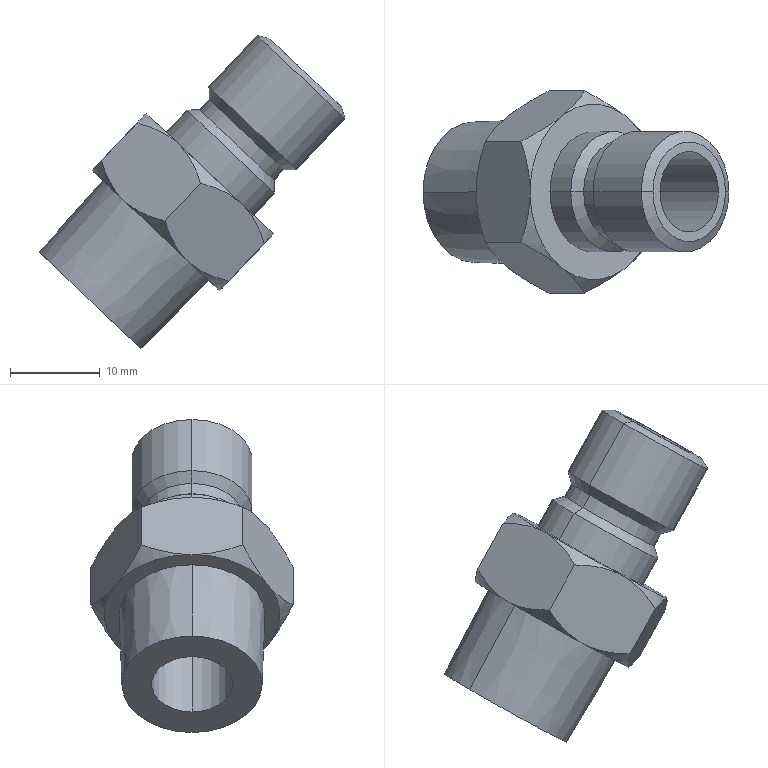Part | STEP file | 4-20.sldasm-Part-51 | 1 solid | 38 faces | box 34.118 x 22.56 x 34.901 mm | volume 4861 mm3 | cone 20 | plane 10 | cylinder 8 | commonest cylinder face diameters 13.462 x4 9 x2 11.43 x2
STEP:
#1=CARTESIAN_POINT('',(267.035,-375.875,53.742));
#2=VERTEX_POINT('',#1);
#3=CARTESIAN_POINT('',(255.664,-375.875,64.491));
#4=VERTEX_POINT('',#3);
#5=CARTESIAN_POINT('',(261.349,-375.875,59.117));
#6=DIRECTION('',(0.687,0.,0.7267));
#7=DIRECTION('',(-0.7267,0.,0.687));
#8=AXIS2_PLACEMENT_3D('',#5,#6,#7);
#9=CIRCLE('',#8,7.824);
#10=EDGE_CURVE('',#2,#4,#9,.T.);
#11=ORIENTED_EDGE('',*,*,#10,.T.);
#12=CARTESIAN_POINT('',(262.798,-375.875,72.445));
#13=VERTEX_POINT('',#12);
#14=CARTESIAN_POINT('',(262.798,-375.875,72.445));
#15=DIRECTION('',(0.6677,0.,0.7444));
#16=VECTOR('',#15,1000.);
#17=LINE('',#14,#16);
#18=EDGE_CURVE('',#4,#13,#17,.T.);
#19=ORIENTED_EDGE('',*,*,#18,.T.);
#20=CARTESIAN_POINT('',(274.575,-375.875,61.312));
#21=VERTEX_POINT('',#20);
#22=CARTESIAN_POINT('',(268.686,-375.875,66.878));
#23=DIRECTION('',(-0.687,0.,-0.7267));
#24=DIRECTION('',(-0.7267,0.,0.687));
#25=AXIS2_PLACEMENT_3D('',#22,#23,#24);
#26=CIRCLE('',#25,8.103);
#27=EDGE_CURVE('',#13,#21,#26,.T.);
#28=ORIENTED_EDGE('',*,*,#27,.T.);
#29=CARTESIAN_POINT('',(274.575,-375.875,61.312));
#30=DIRECTION('',(0.7057,0.,0.7085));
#31=VECTOR('',#30,1000.);
#32=LINE('',#29,#31);
#33=EDGE_CURVE('',#2,#21,#32,.T.);
#34=ORIENTED_EDGE('',*,*,#33,.F.);
#35=EDGE_LOOP('',(#11,#19,#28,#34));
#36=FACE_OUTER_BOUND('',#35,.T.);
#37=CARTESIAN_POINT('',(268.686,-375.875,66.878));
#38=DIRECTION('',(0.687,0.,0.7267));
#39=DIRECTION('',(0.7267,0.,-0.687));
#40=AXIS2_PLACEMENT_3D('',#37,#38,#39);
#41=CONICAL_SURFACE('',#40,8.103,0.02618);
#42=ADVANCED_FACE('',(#36),#41,.T.);
#43=CARTESIAN_POINT('',(289.399,-375.875,80.678));
#44=VERTEX_POINT('',#43);
#45=CARTESIAN_POINT('',(281.301,-375.875,88.334));
#46=VERTEX_POINT('',#45);
#47=CARTESIAN_POINT('',(285.35,-375.875,84.506));
#48=DIRECTION('',(0.687,0.,0.7267));
#49=DIRECTION('',(-0.7267,0.,0.687));
#50=AXIS2_PLACEMENT_3D('',#47,#48,#49);
#51=CIRCLE('',#50,5.572);
#52=EDGE_CURVE('',#44,#46,#51,.T.);
#53=ORIENTED_EDGE('',*,*,#52,.F.);
#54=CARTESIAN_POINT('',(289.781,-375.875,79.396));
#55=VERTEX_POINT('',#54);
#56=CARTESIAN_POINT('',(289.151,-375.875,81.508));
#57=DIRECTION('',(0.2859,0.,-0.9583));
#58=VECTOR('',#57,1000.);
#59=LINE('',#56,#58);
#60=EDGE_CURVE('',#44,#55,#59,.T.);
#61=ORIENTED_EDGE('',*,*,#60,.T.);
#62=CARTESIAN_POINT('',(279.999,-375.875,88.643));
#63=VERTEX_POINT('',#62);
#64=CARTESIAN_POINT('',(284.89,-375.875,84.02));
#65=DIRECTION('',(0.687,0.,0.7267));
#66=DIRECTION('',(-0.7267,0.,0.687));
#67=AXIS2_PLACEMENT_3D('',#64,#65,#66);
#68=CIRCLE('',#67,6.731);
#69=EDGE_CURVE('',#55,#63,#68,.T.);
#70=ORIENTED_EDGE('',*,*,#69,.T.);
#71=CARTESIAN_POINT('',(282.143,-375.875,88.133));
#72=DIRECTION('',(-0.9728,0.,0.2316));
#73=VECTOR('',#72,1000.);
#74=LINE('',#71,#73);
#75=EDGE_CURVE('',#46,#63,#74,.T.);
#76=ORIENTED_EDGE('',*,*,#75,.F.);
#77=EDGE_LOOP('',(#53,#61,#70,#76));
#78=FACE_OUTER_BOUND('',#77,.T.);
#79=CARTESIAN_POINT('',(285.647,-375.875,84.821));
#80=DIRECTION('',(-0.687,0.,-0.7267));
#81=DIRECTION('',(-0.7267,0.,0.687));
#82=AXIS2_PLACEMENT_3D('',#79,#80,#81);
#83=CONICAL_SURFACE('',#82,4.822,1.047);
#84=ADVANCED_FACE('',(#78),#83,.T.);
#85=ORIENTED_EDGE('',*,*,#69,.F.);
#86=CARTESIAN_POINT('',(284.396,-375.875,73.698));
#87=VERTEX_POINT('',#86);
#88=CARTESIAN_POINT('',(266.241,-375.875,54.493));
#89=DIRECTION('',(-0.687,0.,-0.7267));
#90=VECTOR('',#89,1000.);
#91=LINE('',#88,#90);
#92=EDGE_CURVE('',#55,#87,#91,.T.);
#93=ORIENTED_EDGE('',*,*,#92,.T.);
#94=CARTESIAN_POINT('',(274.613,-375.875,82.946));
#95=VERTEX_POINT('',#94);
#96=CARTESIAN_POINT('',(279.504,-375.875,78.322));
#97=DIRECTION('',(0.687,0.,0.7267));
#98=DIRECTION('',(-0.7267,0.,0.687));
#99=AXIS2_PLACEMENT_3D('',#96,#97,#98);
#100=CIRCLE('',#99,6.731);
#101=EDGE_CURVE('',#87,#95,#100,.T.);
#102=ORIENTED_EDGE('',*,*,#101,.T.);
#103=CARTESIAN_POINT('',(256.458,-375.875,63.74));
#104=DIRECTION('',(-0.687,0.,-0.7267));
#105=VECTOR('',#104,1000.);
#106=LINE('',#103,#105);
#107=EDGE_CURVE('',#63,#95,#106,.T.);
#108=ORIENTED_EDGE('',*,*,#107,.F.);
#109=EDGE_LOOP('',(#85,#93,#102,#108));
#110=FACE_OUTER_BOUND('',#109,.T.);
#111=CARTESIAN_POINT('',(261.349,-375.875,59.117));
#112=DIRECTION('',(-0.687,0.,-0.7267));
#113=DIRECTION('',(-0.7267,0.,0.687));
#114=AXIS2_PLACEMENT_3D('',#111,#112,#113);
#115=CYLINDRICAL_SURFACE('',#114,6.731);
#116=ADVANCED_FACE('',(#110),#115,.T.);
#117=CARTESIAN_POINT('',(282.96,-375.875,73.658));
#118=VERTEX_POINT('',#117);
#119=CARTESIAN_POINT('',(274.653,-375.875,81.51));
#120=VERTEX_POINT('',#119);
#121=CARTESIAN_POINT('',(278.806,-375.875,77.584));
#122=DIRECTION('',(0.687,0.,0.7267));
#123=DIRECTION('',(-0.7267,0.,0.687));
#124=AXIS2_PLACEMENT_3D('',#121,#122,#123);
#125=CIRCLE('',#124,5.715);
#126=EDGE_CURVE('',#118,#120,#125,.T.);
#127=ORIENTED_EDGE('',*,*,#126,.T.);
#128=CARTESIAN_POINT('',(274.613,-375.875,82.946));
#129=DIRECTION('',(-0.02811,0.,0.9996));
#130=VECTOR('',#129,1000.);
#131=LINE('',#128,#130);
#132=EDGE_CURVE('',#120,#95,#131,.T.);
#133=ORIENTED_EDGE('',*,*,#132,.T.);
#134=ORIENTED_EDGE('',*,*,#101,.F.);
#135=CARTESIAN_POINT('',(284.396,-375.875,73.698));
#136=DIRECTION('',(0.9996,0.,0.02811));
#137=VECTOR('',#136,1000.);
#138=LINE('',#135,#137);
#139=EDGE_CURVE('',#118,#87,#138,.T.);
#140=ORIENTED_EDGE('',*,*,#139,.F.);
#141=EDGE_LOOP('',(#127,#133,#134,#140));
#142=FACE_OUTER_BOUND('',#141,.T.);
#143=CARTESIAN_POINT('',(279.504,-375.875,78.322));
#144=DIRECTION('',(0.687,0.,0.7267));
#145=DIRECTION('',(0.7267,0.,-0.687));
#146=AXIS2_PLACEMENT_3D('',#143,#144,#145);
#147=CONICAL_SURFACE('',#146,6.731,0.7854);
#148=ADVANCED_FACE('',(#142),#147,.T.);
#149=ORIENTED_EDGE('',*,*,#126,.F.);
#150=CARTESIAN_POINT('',(281.878,-375.875,72.514));
#151=VERTEX_POINT('',#150);
#152=CARTESIAN_POINT('',(265.502,-375.875,55.191));
#153=DIRECTION('',(-0.687,0.,-0.7267));
#154=VECTOR('',#153,1000.);
#155=LINE('',#152,#154);
#156=EDGE_CURVE('',#118,#151,#155,.T.);
#157=ORIENTED_EDGE('',*,*,#156,.T.);
#158=CARTESIAN_POINT('',(273.572,-375.875,80.366));
#159=VERTEX_POINT('',#158);
#160=CARTESIAN_POINT('',(277.725,-375.875,76.44));
#161=DIRECTION('',(0.687,0.,0.7267));
#162=DIRECTION('',(-0.7267,0.,0.687));
#163=AXIS2_PLACEMENT_3D('',#160,#161,#162);
#164=CIRCLE('',#163,5.715);
#165=EDGE_CURVE('',#151,#159,#164,.T.);
#166=ORIENTED_EDGE('',*,*,#165,.T.);
#167=CARTESIAN_POINT('',(257.196,-375.875,63.043));
#168=DIRECTION('',(-0.687,0.,-0.7267));
#169=VECTOR('',#168,1000.);
#170=LINE('',#167,#169);
#171=EDGE_CURVE('',#120,#159,#170,.T.);
#172=ORIENTED_EDGE('',*,*,#171,.F.);
#173=EDGE_LOOP('',(#149,#157,#166,#172));
#174=FACE_OUTER_BOUND('',#173,.T.);
#175=CARTESIAN_POINT('',(261.349,-375.875,59.117));
#176=DIRECTION('',(-0.687,0.,-0.7267));
#177=DIRECTION('',(-0.7267,0.,0.687));
#178=AXIS2_PLACEMENT_3D('',#175,#176,#177);
#179=CYLINDRICAL_SURFACE('',#178,5.715);
#180=ADVANCED_FACE('',(#174),#179,.T.);
#181=ORIENTED_EDGE('',*,*,#165,.F.);
#182=CARTESIAN_POINT('',(281.918,-375.875,71.077));
#183=VERTEX_POINT('',#182);
#184=CARTESIAN_POINT('',(281.878,-375.875,72.514));
#185=DIRECTION('',(0.02811,0.,-0.9996));
#186=VECTOR('',#185,1000.);
#187=LINE('',#184,#186);
#188=EDGE_CURVE('',#151,#183,#187,.T.);
#189=ORIENTED_EDGE('',*,*,#188,.T.);
#190=CARTESIAN_POINT('',(272.135,-375.875,80.325));
#191=VERTEX_POINT('',#190);
#192=CARTESIAN_POINT('',(277.027,-375.875,75.701));
#193=DIRECTION('',(0.687,0.,0.7267));
#194=DIRECTION('',(-0.7267,0.,0.687));
#195=AXIS2_PLACEMENT_3D('',#192,#193,#194);
#196=CIRCLE('',#195,6.731);
#197=EDGE_CURVE('',#183,#191,#196,.T.);
#198=ORIENTED_EDGE('',*,*,#197,.T.);
#199=CARTESIAN_POINT('',(273.572,-375.875,80.366));
#200=DIRECTION('',(-0.9996,0.,-0.02811));
#201=VECTOR('',#200,1000.);
#202=LINE('',#199,#201);
#203=EDGE_CURVE('',#159,#191,#202,.T.);
#204=ORIENTED_EDGE('',*,*,#203,.F.);
#205=EDGE_LOOP('',(#181,#189,#198,#204));
#206=FACE_OUTER_BOUND('',#205,.T.);
#207=CARTESIAN_POINT('',(277.725,-375.875,76.44));
#208=DIRECTION('',(-0.687,0.,-0.7267));
#209=DIRECTION('',(-0.7267,0.,0.687));
#210=AXIS2_PLACEMENT_3D('',#207,#208,#209);
#211=CONICAL_SURFACE('',#210,5.715,0.7854);
#212=ADVANCED_FACE('',(#206),#211,.T.);
#213=ORIENTED_EDGE('',*,*,#197,.F.);
#214=CARTESIAN_POINT('',(279.598,-375.875,68.622));
#215=VERTEX_POINT('',#214);
#216=CARTESIAN_POINT('',(266.241,-375.875,54.493));
#217=DIRECTION('',(-0.687,0.,-0.7267));
#218=VECTOR('',#217,1000.);
#219=LINE('',#216,#218);
#220=EDGE_CURVE('',#183,#215,#219,.T.);
#221=ORIENTED_EDGE('',*,*,#220,.T.);
#222=CARTESIAN_POINT('',(269.815,-375.875,77.87));
#223=VERTEX_POINT('',#222);
#224=CARTESIAN_POINT('',(274.706,-375.875,73.246));
#225=DIRECTION('',(0.687,0.,0.7267));
#226=DIRECTION('',(-0.7267,0.,0.687));
#227=AXIS2_PLACEMENT_3D('',#224,#225,#226);
#228=CIRCLE('',#227,6.731);
#229=EDGE_CURVE('',#215,#223,#228,.T.);
#230=ORIENTED_EDGE('',*,*,#229,.T.);
#231=CARTESIAN_POINT('',(256.458,-375.875,63.74));
#232=DIRECTION('',(-0.687,0.,-0.7267));
#233=VECTOR('',#232,1000.);
#234=LINE('',#231,#233);
#235=EDGE_CURVE('',#191,#223,#234,.T.);
#236=ORIENTED_EDGE('',*,*,#235,.F.);
#237=EDGE_LOOP('',(#213,#221,#230,#236));
#238=FACE_OUTER_BOUND('',#237,.T.);
#239=CARTESIAN_POINT('',(261.349,-375.875,59.117));
#240=DIRECTION('',(-0.687,0.,-0.7267));
#241=DIRECTION('',(-0.7267,0.,0.687));
#242=AXIS2_PLACEMENT_3D('',#239,#240,#241);
#243=CYLINDRICAL_SURFACE('',#242,6.731);
#244=ADVANCED_FACE('',(#238),#243,.T.);
#245=CARTESIAN_POINT('',(264.619,-375.875,56.025));
#246=VERTEX_POINT('',#245);
#247=CARTESIAN_POINT('',(258.079,-375.875,62.208));
#248=VERTEX_POINT('',#247);
#249=CARTESIAN_POINT('',(261.349,-375.875,59.117));
#250=DIRECTION('',(-0.687,0.,-0.7267));
#251=DIRECTION('',(-0.7267,0.,0.687));
#252=AXIS2_PLACEMENT_3D('',#249,#250,#251);
#253=CIRCLE('',#252,4.5);
#254=EDGE_CURVE('',#246,#248,#253,.T.);
#255=ORIENTED_EDGE('',*,*,#254,.T.);
#256=CARTESIAN_POINT('',(282.08,-375.875,87.597));
#257=VERTEX_POINT('',#256);
#258=CARTESIAN_POINT('',(13.738,-375.875,-196.272));
#259=DIRECTION('',(0.687,0.,0.7267));
#260=VECTOR('',#259,1000.);
#261=LINE('',#258,#260);
#262=EDGE_CURVE('',#248,#257,#261,.T.);
#263=ORIENTED_EDGE('',*,*,#262,.T.);
#264=CARTESIAN_POINT('',(288.62,-375.875,81.415));
#265=VERTEX_POINT('',#264);
#266=CARTESIAN_POINT('',(285.35,-375.875,84.506));
#267=DIRECTION('',(-0.687,0.,-0.7267));
#268=DIRECTION('',(-0.6293,-0.5,0.5949));
#269=AXIS2_PLACEMENT_3D('',#266,#267,#268);
#270=CIRCLE('',#269,4.5);
#271=EDGE_CURVE('',#265,#257,#270,.T.);
#272=ORIENTED_EDGE('',*,*,#271,.F.);
#273=CARTESIAN_POINT('',(20.278,-375.875,-202.454));
#274=DIRECTION('',(0.687,0.,0.7267));
#275=VECTOR('',#274,1000.);
#276=LINE('',#273,#275);
#277=EDGE_CURVE('',#246,#265,#276,.T.);
#278=ORIENTED_EDGE('',*,*,#277,.F.);
#279=EDGE_LOOP('',(#255,#263,#272,#278));
#280=FACE_OUTER_BOUND('',#279,.T.);
#281=CARTESIAN_POINT('',(17.008,-375.875,-199.363));
#282=DIRECTION('',(0.687,0.,0.7267));
#283=DIRECTION('',(0.7267,0.,-0.687));
#284=AXIS2_PLACEMENT_3D('',#281,#282,#283);
#285=CYLINDRICAL_SURFACE('',#284,4.5);
#286=ADVANCED_FACE('',(#280),#285,.F.);
#287=CARTESIAN_POINT('',(261.587,-375.406,73.589));
#288=VERTEX_POINT('',#287);
#289=CARTESIAN_POINT('',(261.587,-376.344,73.589));
#290=VERTEX_POINT('',#289);
#291=CARTESIAN_POINT('',(261.587,-370.235,73.589));
#292=DIRECTION('',(0.,-1.,0.));
#293=VECTOR('',#292,1000.);
#294=LINE('',#291,#293);
#295=EDGE_CURVE('',#288,#290,#294,.T.);
#296=ORIENTED_EDGE('',*,*,#295,.F.);
#297=CARTESIAN_POINT('',(264.842,-367.649,70.512));
#298=VERTEX_POINT('',#297);
#299=CARTESIAN_POINT('',(268.686,-375.875,66.878));
#300=DIRECTION('',(0.687,0.,0.7267));
#301=DIRECTION('',(-0.7267,0.,0.687));
#302=AXIS2_PLACEMENT_3D('',#299,#300,#301);
#303=CIRCLE('',#302,9.78);
#304=EDGE_CURVE('',#298,#288,#303,.T.);
#305=ORIENTED_EDGE('',*,*,#304,.F.);
#306=CARTESIAN_POINT('',(265.432,-367.181,69.955));
#307=VERTEX_POINT('',#306);
#308=CARTESIAN_POINT('',(268.686,-364.595,66.878));
#309=DIRECTION('',(-0.6293,-0.5,0.5949));
#310=VECTOR('',#309,1000.);
#311=LINE('',#308,#310);
#312=EDGE_CURVE('',#307,#298,#311,.T.);
#313=ORIENTED_EDGE('',*,*,#312,.F.);
#314=CARTESIAN_POINT('',(271.941,-367.181,63.802));
#315=VERTEX_POINT('',#314);
#316=CARTESIAN_POINT('',(268.686,-375.875,66.878));
#317=DIRECTION('',(0.687,0.,0.7267));
#318=DIRECTION('',(-0.7267,0.,0.687));
#319=AXIS2_PLACEMENT_3D('',#316,#317,#318);
#320=CIRCLE('',#319,9.78);
#321=EDGE_CURVE('',#315,#307,#320,.T.);
#322=ORIENTED_EDGE('',*,*,#321,.F.);
#323=CARTESIAN_POINT('',(272.531,-367.649,63.244));
#324=VERTEX_POINT('',#323);
#325=CARTESIAN_POINT('',(275.785,-370.235,60.168));
#326=DIRECTION('',(-0.6293,0.5,0.5949));
#327=VECTOR('',#326,1000.);
#328=LINE('',#325,#327);
#329=EDGE_CURVE('',#324,#315,#328,.T.);
#330=ORIENTED_EDGE('',*,*,#329,.F.);
#331=CARTESIAN_POINT('',(275.785,-375.406,60.168));
#332=VERTEX_POINT('',#331);
#333=CARTESIAN_POINT('',(268.686,-375.875,66.878));
#334=DIRECTION('',(0.687,0.,0.7267));
#335=DIRECTION('',(-0.7267,0.,0.687));
#336=AXIS2_PLACEMENT_3D('',#333,#334,#335);
#337=CIRCLE('',#336,9.78);
#338=EDGE_CURVE('',#332,#324,#337,.T.);
#339=ORIENTED_EDGE('',*,*,#338,.F.);
#340=CARTESIAN_POINT('',(275.785,-376.344,60.168));
#341=VERTEX_POINT('',#340);
#342=CARTESIAN_POINT('',(275.785,-381.515,60.168));
#343=DIRECTION('',(0.,1.,0.));
#344=VECTOR('',#343,1000.);
#345=LINE('',#342,#344);
#346=EDGE_CURVE('',#341,#332,#345,.T.);
#347=ORIENTED_EDGE('',*,*,#346,.F.);
#348=CARTESIAN_POINT('',(272.531,-384.101,63.244));
#349=VERTEX_POINT('',#348);
#350=CARTESIAN_POINT('',(268.686,-375.875,66.878));
#351=DIRECTION('',(0.687,0.,0.7267));
#352=DIRECTION('',(-0.7267,0.,0.687));
#353=AXIS2_PLACEMENT_3D('',#350,#351,#352);
#354=CIRCLE('',#353,9.78);
#355=EDGE_CURVE('',#349,#341,#354,.T.);
#356=ORIENTED_EDGE('',*,*,#355,.F.);
#357=CARTESIAN_POINT('',(271.941,-384.569,63.802));
#358=VERTEX_POINT('',#357);
#359=CARTESIAN_POINT('',(268.686,-387.155,66.878));
#360=DIRECTION('',(0.6293,0.5,-0.5949));
#361=VECTOR('',#360,1000.);
#362=LINE('',#359,#361);
#363=EDGE_CURVE('',#358,#349,#362,.T.);
#364=ORIENTED_EDGE('',*,*,#363,.F.);
#365=CARTESIAN_POINT('',(265.432,-384.569,69.955));
#366=VERTEX_POINT('',#365);
#367=CARTESIAN_POINT('',(268.686,-375.875,66.878));
#368=DIRECTION('',(0.687,0.,0.7267));
#369=DIRECTION('',(-0.7267,0.,0.687));
#370=AXIS2_PLACEMENT_3D('',#367,#368,#369);
#371=CIRCLE('',#370,9.78);
#372=EDGE_CURVE('',#366,#358,#371,.T.);
#373=ORIENTED_EDGE('',*,*,#372,.F.);
#374=CARTESIAN_POINT('',(264.842,-384.101,70.512));
#375=VERTEX_POINT('',#374);
#376=CARTESIAN_POINT('',(261.587,-381.515,73.589));
#377=DIRECTION('',(0.6293,-0.5,-0.5949));
#378=VECTOR('',#377,1000.);
#379=LINE('',#376,#378);
#380=EDGE_CURVE('',#375,#366,#379,.T.);
#381=ORIENTED_EDGE('',*,*,#380,.F.);
#382=CARTESIAN_POINT('',(268.686,-375.875,66.878));
#383=DIRECTION('',(0.687,0.,0.7267));
#384=DIRECTION('',(-0.7267,0.,0.687));
#385=AXIS2_PLACEMENT_3D('',#382,#383,#384);
#386=CIRCLE('',#385,9.78);
#387=EDGE_CURVE('',#290,#375,#386,.T.);
#388=ORIENTED_EDGE('',*,*,#387,.F.);
#389=EDGE_LOOP('',(#296,#305,#313,#322,#330,#339,#347,#356,#364,#373,#381,#388));
#390=FACE_OUTER_BOUND('',#389,.T.);
#391=CARTESIAN_POINT('',(268.686,-375.875,66.878));
#392=DIRECTION('',(-0.687,0.,-0.7267));
#393=DIRECTION('',(-0.7267,0.,0.687));
#394=AXIS2_PLACEMENT_3D('',#391,#392,#393);
#395=CIRCLE('',#394,8.103);
#396=EDGE_CURVE('',#21,#13,#395,.T.);
#397=ORIENTED_EDGE('',*,*,#396,.F.);
#398=ORIENTED_EDGE('',*,*,#27,.F.);
#399=EDGE_LOOP('',(#397,#398));
#400=FACE_BOUND('',#399,.T.);
#401=CARTESIAN_POINT('',(268.686,-375.875,66.878));
#402=DIRECTION('',(-0.687,0.,-0.7267));
#403=DIRECTION('',(-0.7267,0.,0.687));
#404=AXIS2_PLACEMENT_3D('',#401,#402,#403);
#405=PLANE('',#404);
#406=ADVANCED_FACE('',(#390,#400),#405,.T.);
#407=ORIENTED_EDGE('',*,*,#262,.F.);
#408=CARTESIAN_POINT('',(261.349,-375.875,59.117));
#409=DIRECTION('',(-0.687,0.,-0.7267));
#410=DIRECTION('',(-0.7267,0.,0.687));
#411=AXIS2_PLACEMENT_3D('',#408,#409,#410);
#412=CIRCLE('',#411,4.5);
#413=EDGE_CURVE('',#248,#246,#412,.T.);
#414=ORIENTED_EDGE('',*,*,#413,.T.);
#415=ORIENTED_EDGE('',*,*,#277,.T.);
#416=CARTESIAN_POINT('',(285.35,-375.875,84.506));
#417=DIRECTION('',(-0.687,0.,-0.7267));
#418=DIRECTION('',(-0.6293,-0.5,0.5949));
#419=AXIS2_PLACEMENT_3D('',#416,#417,#418);
#420=CIRCLE('',#419,4.5);
#421=EDGE_CURVE('',#257,#265,#420,.T.);
#422=ORIENTED_EDGE('',*,*,#421,.F.);
#423=EDGE_LOOP('',(#407,#414,#415,#422));
#424=FACE_OUTER_BOUND('',#423,.T.);
#425=CARTESIAN_POINT('',(17.008,-375.875,-199.363));
#426=DIRECTION('',(0.687,0.,0.7267));
#427=DIRECTION('',(0.7267,0.,-0.687));
#428=AXIS2_PLACEMENT_3D('',#425,#426,#427);
#429=CYLINDRICAL_SURFACE('',#428,4.5);
#430=ADVANCED_FACE('',(#424),#429,.F.);
#431=CARTESIAN_POINT('',(285.35,-375.875,84.506));
#432=DIRECTION('',(0.687,0.,0.7267));
#433=DIRECTION('',(-0.7267,0.,0.687));
#434=AXIS2_PLACEMENT_3D('',#431,#432,#433);
#435=CIRCLE('',#434,5.572);
#436=EDGE_CURVE('',#46,#44,#435,.T.);
#437=ORIENTED_EDGE('',*,*,#436,.T.);
#438=ORIENTED_EDGE('',*,*,#52,.T.);
#439=EDGE_LOOP('',(#437,#438));
#440=FACE_OUTER_BOUND('',#439,.T.);
#441=ORIENTED_EDGE('',*,*,#271,.T.);
#442=ORIENTED_EDGE('',*,*,#421,.T.);
#443=EDGE_LOOP('',(#441,#442));
#444=FACE_BOUND('',#443,.T.);
#445=CARTESIAN_POINT('',(285.35,-375.875,84.506));
#446=DIRECTION('',(-0.687,0.,-0.7267));
#447=DIRECTION('',(-0.7267,0.,0.687));
#448=AXIS2_PLACEMENT_3D('',#445,#446,#447);
#449=PLANE('',#448);
#450=ADVANCED_FACE('',(#440,#444),#449,.F.);
#451=CARTESIAN_POINT('',(270.862,-384.101,76.88));
#452=VERTEX_POINT('',#451);
#453=CARTESIAN_POINT('',(266.577,-381.515,78.867));
#454=VERTEX_POINT('',#453);
#455=CARTESIAN_POINT('',(270.862,-384.101,76.88));
#456=CARTESIAN_POINT('',(270.561,-383.874,77.135));
#457=CARTESIAN_POINT('',(270.239,-383.647,77.365));
#458=CARTESIAN_POINT('',(269.569,-383.204,77.775));
#459=CARTESIAN_POINT('',(269.219,-382.985,77.956));
#460=CARTESIAN_POINT('',(268.495,-382.553,78.278));
#461=CARTESIAN_POINT('',(268.118,-382.339,78.42));
#462=CARTESIAN_POINT('',(267.354,-381.92,78.668));
#463=CARTESIAN_POINT('',(266.967,-381.716,78.774));
#464=CARTESIAN_POINT('',(266.577,-381.515,78.867));
#465=B_SPLINE_CURVE_WITH_KNOTS('',3,(#455,#456,#457,#458,#459,#460,#461,#462,#463,#464),.UNSPECIFIED.,.F.,.F.,(4,2,2,2,4),(0.01592,0.01727,0.01863,0.01998,0.02133),.UNSPECIFIED.);
#466=EDGE_CURVE('',#452,#454,#465,.T.);
#467=ORIENTED_EDGE('',*,*,#466,.F.);
#468=CARTESIAN_POINT('',(267.607,-376.344,79.957));
#469=VERTEX_POINT('',#468);
#470=CARTESIAN_POINT('',(274.706,-375.875,73.246));
#471=DIRECTION('',(-0.687,0.,-0.7267));
#472=DIRECTION('',(-0.7267,0.,0.687));
#473=AXIS2_PLACEMENT_3D('',#470,#471,#472);
#474=CIRCLE('',#473,9.78);
#475=EDGE_CURVE('',#452,#469,#474,.T.);
#476=ORIENTED_EDGE('',*,*,#475,.T.);
#477=CARTESIAN_POINT('',(266.577,-381.515,78.867));
#478=CARTESIAN_POINT('',(266.716,-381.11,79.014));
#479=CARTESIAN_POINT('',(266.846,-380.697,79.152));
#480=CARTESIAN_POINT('',(267.082,-379.861,79.402));
#481=CARTESIAN_POINT('',(267.188,-379.438,79.514));
#482=CARTESIAN_POINT('',(267.369,-378.577,79.705));
#483=CARTESIAN_POINT('',(267.443,-378.14,79.784));
#484=CARTESIAN_POINT('',(267.556,-377.248,79.903));
#485=CARTESIAN_POINT('',(267.592,-376.793,79.941));
#486=CARTESIAN_POINT('',(267.607,-376.344,79.957));
#487=B_SPLINE_CURVE_WITH_KNOTS('',3,(#477,#478,#479,#480,#481,#482,#483,#484,#485,#486),.UNSPECIFIED.,.F.,.F.,(4,2,2,2,4),(0.00821,0.009558,0.01091,0.01225,0.0136),.UNSPECIFIED.);
#488=EDGE_CURVE('',#454,#469,#487,.T.);
#489=ORIENTED_EDGE('',*,*,#488,.F.);
#490=EDGE_LOOP('',(#467,#476,#489));
#491=FACE_OUTER_BOUND('',#490,.T.);
#492=CARTESIAN_POINT('',(274.706,-375.875,73.246));
#493=DIRECTION('',(-0.687,0.,-0.7267));
#494=DIRECTION('',(-0.7267,0.,0.687));
#495=AXIS2_PLACEMENT_3D('',#492,#493,#494);
#496=CONICAL_SURFACE('',#495,9.78,0.7854);
#497=ADVANCED_FACE('',(#491),#496,.T.);
#498=CARTESIAN_POINT('',(274.706,-375.875,73.246));
#499=DIRECTION('',(0.687,0.,0.7267));
#500=DIRECTION('',(-0.7267,0.,0.687));
#501=AXIS2_PLACEMENT_3D('',#498,#499,#500);
#502=CIRCLE('',#501,6.731);
#503=EDGE_CURVE('',#223,#215,#502,.T.);
#504=ORIENTED_EDGE('',*,*,#503,.F.);
#505=ORIENTED_EDGE('',*,*,#229,.F.);
#506=EDGE_LOOP('',(#504,#505));
#507=FACE_BOUND('',#506,.T.);
#508=CARTESIAN_POINT('',(267.607,-375.406,79.957));
#509=VERTEX_POINT('',#508);
#510=CARTESIAN_POINT('',(267.607,-370.235,79.957));
#511=DIRECTION('',(0.,-1.,0.));
#512=VECTOR('',#511,1000.);
#513=LINE('',#510,#512);
#514=EDGE_CURVE('',#509,#469,#513,.T.);
#515=ORIENTED_EDGE('',*,*,#514,.T.);
#516=ORIENTED_EDGE('',*,*,#475,.F.);
#517=CARTESIAN_POINT('',(271.452,-384.569,76.323));
#518=VERTEX_POINT('',#517);
#519=CARTESIAN_POINT('',(267.607,-381.515,79.957));
#520=DIRECTION('',(0.6293,-0.5,-0.5949));
#521=VECTOR('',#520,1000.);
#522=LINE('',#519,#521);
#523=EDGE_CURVE('',#452,#518,#522,.T.);
#524=ORIENTED_EDGE('',*,*,#523,.T.);
#525=CARTESIAN_POINT('',(277.961,-384.569,70.17));
#526=VERTEX_POINT('',#525);
#527=CARTESIAN_POINT('',(274.706,-375.875,73.246));
#528=DIRECTION('',(-0.687,0.,-0.7267));
#529=DIRECTION('',(-0.7267,0.,0.687));
#530=AXIS2_PLACEMENT_3D('',#527,#528,#529);
#531=CIRCLE('',#530,9.78);
#532=EDGE_CURVE('',#526,#518,#531,.T.);
#533=ORIENTED_EDGE('',*,*,#532,.F.);
#534=CARTESIAN_POINT('',(278.55,-384.101,69.612));
#535=VERTEX_POINT('',#534);
#536=CARTESIAN_POINT('',(274.706,-387.155,73.246));
#537=DIRECTION('',(0.6293,0.5,-0.5949));
#538=VECTOR('',#537,1000.);
#539=LINE('',#536,#538);
#540=EDGE_CURVE('',#526,#535,#539,.T.);
#541=ORIENTED_EDGE('',*,*,#540,.T.);
#542=CARTESIAN_POINT('',(281.805,-376.344,66.536));
#543=VERTEX_POINT('',#542);
#544=CARTESIAN_POINT('',(274.706,-375.875,73.246));
#545=DIRECTION('',(-0.687,0.,-0.7267));
#546=DIRECTION('',(-0.7267,0.,0.687));
#547=AXIS2_PLACEMENT_3D('',#544,#545,#546);
#548=CIRCLE('',#547,9.78);
#549=EDGE_CURVE('',#543,#535,#548,.T.);
#550=ORIENTED_EDGE('',*,*,#549,.F.);
#551=CARTESIAN_POINT('',(281.805,-375.406,66.536));
#552=VERTEX_POINT('',#551);
#553=CARTESIAN_POINT('',(281.805,-381.515,66.536));
#554=DIRECTION('',(0.,1.,0.));
#555=VECTOR('',#554,1000.);
#556=LINE('',#553,#555);
#557=EDGE_CURVE('',#543,#552,#556,.T.);
#558=ORIENTED_EDGE('',*,*,#557,.T.);
#559=CARTESIAN_POINT('',(278.55,-367.649,69.612));
#560=VERTEX_POINT('',#559);
#561=CARTESIAN_POINT('',(274.706,-375.875,73.246));
#562=DIRECTION('',(-0.687,0.,-0.7267));
#563=DIRECTION('',(-0.7267,0.,0.687));
#564=AXIS2_PLACEMENT_3D('',#561,#562,#563);
#565=CIRCLE('',#564,9.78);
#566=EDGE_CURVE('',#560,#552,#565,.T.);
#567=ORIENTED_EDGE('',*,*,#566,.F.);
#568=CARTESIAN_POINT('',(277.961,-367.181,70.17));
#569=VERTEX_POINT('',#568);
#570=CARTESIAN_POINT('',(281.805,-370.235,66.536));
#571=DIRECTION('',(-0.6293,0.5,0.5949));
#572=VECTOR('',#571,1000.);
#573=LINE('',#570,#572);
#574=EDGE_CURVE('',#560,#569,#573,.T.);
#575=ORIENTED_EDGE('',*,*,#574,.T.);
#576=CARTESIAN_POINT('',(271.452,-367.181,76.323));
#577=VERTEX_POINT('',#576);
#578=CARTESIAN_POINT('',(274.706,-375.875,73.246));
#579=DIRECTION('',(-0.687,0.,-0.7267));
#580=DIRECTION('',(-0.7267,0.,0.687));
#581=AXIS2_PLACEMENT_3D('',#578,#579,#580);
#582=CIRCLE('',#581,9.78);
#583=EDGE_CURVE('',#577,#569,#582,.T.);
#584=ORIENTED_EDGE('',*,*,#583,.F.);
#585=CARTESIAN_POINT('',(270.862,-367.649,76.88));
#586=VERTEX_POINT('',#585);
#587=CARTESIAN_POINT('',(274.706,-364.595,73.246));
#588=DIRECTION('',(-0.6293,-0.5,0.5949));
#589=VECTOR('',#588,1000.);
#590=LINE('',#587,#589);
#591=EDGE_CURVE('',#577,#586,#590,.T.);
#592=ORIENTED_EDGE('',*,*,#591,.T.);
#593=CARTESIAN_POINT('',(274.706,-375.875,73.246));
#594=DIRECTION('',(-0.687,0.,-0.7267));
#595=DIRECTION('',(-0.7267,0.,0.687));
#596=AXIS2_PLACEMENT_3D('',#593,#594,#595);
#597=CIRCLE('',#596,9.78);
#598=EDGE_CURVE('',#509,#586,#597,.T.);
#599=ORIENTED_EDGE('',*,*,#598,.F.);
#600=EDGE_LOOP('',(#515,#516,#524,#533,#541,#550,#558,#567,#575,#584,#592,#599));
#601=FACE_OUTER_BOUND('',#600,.T.);
#602=CARTESIAN_POINT('',(274.706,-375.875,73.246));
#603=DIRECTION('',(-0.687,0.,-0.7267));
#604=DIRECTION('',(-0.7267,0.,0.687));
#605=AXIS2_PLACEMENT_3D('',#602,#603,#604);
#606=PLANE('',#605);
#607=ADVANCED_FACE('',(#507,#601),#606,.F.);
#608=CARTESIAN_POINT('',(269.717,-387.155,67.968));
#609=VERTEX_POINT('',#608);
#610=CARTESIAN_POINT('',(269.717,-387.155,67.968));
#611=CARTESIAN_POINT('',(269.948,-386.751,67.193));
#612=CARTESIAN_POINT('',(270.229,-386.335,66.443));
#613=CARTESIAN_POINT('',(270.776,-385.684,65.379));
#614=CARTESIAN_POINT('',(270.979,-385.462,65.035));
#615=CARTESIAN_POINT('',(271.427,-385.018,64.389));
#616=CARTESIAN_POINT('',(271.672,-384.794,64.085));
#617=CARTESIAN_POINT('',(271.941,-384.569,63.802));
#618=B_SPLINE_CURVE_WITH_KNOTS('',3,(#610,#611,#612,#613,#614,#615,#616,#617),.UNSPECIFIED.,.F.,.F.,(4,2,2,4),(0.009563,0.01227,0.01363,0.01498),.UNSPECIFIED.);
#619=EDGE_CURVE('',#609,#358,#618,.T.);
#620=ORIENTED_EDGE('',*,*,#619,.T.);
#621=ORIENTED_EDGE('',*,*,#363,.T.);
#622=CARTESIAN_POINT('',(276.816,-381.515,61.258));
#623=VERTEX_POINT('',#622);
#624=CARTESIAN_POINT('',(272.531,-384.101,63.244));
#625=CARTESIAN_POINT('',(272.831,-383.874,62.99));
#626=CARTESIAN_POINT('',(273.153,-383.647,62.759));
#627=CARTESIAN_POINT('',(273.823,-383.204,62.35));
#628=CARTESIAN_POINT('',(274.173,-382.985,62.169));
#629=CARTESIAN_POINT('',(274.898,-382.553,61.846));
#630=CARTESIAN_POINT('',(275.274,-382.339,61.705));
#631=CARTESIAN_POINT('',(276.038,-381.92,61.457));
#632=CARTESIAN_POINT('',(276.425,-381.716,61.351));
#633=CARTESIAN_POINT('',(276.816,-381.515,61.258));
#634=B_SPLINE_CURVE_WITH_KNOTS('',3,(#624,#625,#626,#627,#628,#629,#630,#631,#632,#633),.UNSPECIFIED.,.F.,.F.,(4,2,2,2,4),(0.01592,0.01727,0.01863,0.01998,0.02133),.UNSPECIFIED.);
#635=EDGE_CURVE('',#349,#623,#634,.T.);
#636=ORIENTED_EDGE('',*,*,#635,.T.);
#637=CARTESIAN_POINT('',(280.775,-381.515,65.446));
#638=VERTEX_POINT('',#637);
#639=CARTESIAN_POINT('',(222.209,-381.515,3.492));
#640=DIRECTION('',(0.687,0.,0.7267));
#641=VECTOR('',#640,1000.);
#642=LINE('',#639,#641);
#643=EDGE_CURVE('',#623,#638,#642,.T.);
#644=ORIENTED_EDGE('',*,*,#643,.T.);
#645=CARTESIAN_POINT('',(280.775,-381.515,65.446));
#646=CARTESIAN_POINT('',(280.543,-381.919,66.221));
#647=CARTESIAN_POINT('',(280.262,-382.335,66.971));
#648=CARTESIAN_POINT('',(279.716,-382.986,68.035));
#649=CARTESIAN_POINT('',(279.512,-383.208,68.379));
#650=CARTESIAN_POINT('',(279.064,-383.652,69.025));
#651=CARTESIAN_POINT('',(278.819,-383.876,69.329));
#652=CARTESIAN_POINT('',(278.55,-384.101,69.612));
#653=B_SPLINE_CURVE_WITH_KNOTS('',3,(#645,#646,#647,#648,#649,#650,#651,#652),.UNSPECIFIED.,.F.,.F.,(4,2,2,4),(0.009563,0.01227,0.01363,0.01498),.UNSPECIFIED.);
#654=EDGE_CURVE('',#638,#535,#653,.T.);
#655=ORIENTED_EDGE('',*,*,#654,.T.);
#656=ORIENTED_EDGE('',*,*,#540,.F.);
#657=CARTESIAN_POINT('',(273.676,-387.155,72.156));
#658=VERTEX_POINT('',#657);
#659=CARTESIAN_POINT('',(277.961,-384.569,70.17));
#660=CARTESIAN_POINT('',(277.66,-384.796,70.424));
#661=CARTESIAN_POINT('',(277.338,-385.023,70.654));
#662=CARTESIAN_POINT('',(276.668,-385.466,71.064));
#663=CARTESIAN_POINT('',(276.318,-385.685,71.245));
#664=CARTESIAN_POINT('',(275.594,-386.117,71.568));
#665=CARTESIAN_POINT('',(275.217,-386.331,71.709));
#666=CARTESIAN_POINT('',(274.453,-386.75,71.957));
#667=CARTESIAN_POINT('',(274.066,-386.954,72.063));
#668=CARTESIAN_POINT('',(273.676,-387.155,72.156));
#669=B_SPLINE_CURVE_WITH_KNOTS('',3,(#659,#660,#661,#662,#663,#664,#665,#666,#667,#668),.UNSPECIFIED.,.F.,.F.,(4,2,2,2,4),(0.01592,0.01727,0.01863,0.01998,0.02133),.UNSPECIFIED.);
#670=EDGE_CURVE('',#526,#658,#669,.T.);
#671=ORIENTED_EDGE('',*,*,#670,.T.);
#672=CARTESIAN_POINT('',(215.11,-387.155,10.202));
#673=DIRECTION('',(0.687,0.,0.7267));
#674=VECTOR('',#673,1000.);
#675=LINE('',#672,#674);
#676=EDGE_CURVE('',#609,#658,#675,.T.);
#677=ORIENTED_EDGE('',*,*,#676,.F.);
#678=EDGE_LOOP('',(#620,#621,#636,#644,#655,#656,#671,#677));
#679=FACE_OUTER_BOUND('',#678,.T.);
#680=CARTESIAN_POINT('',(215.11,-387.155,10.202));
#681=DIRECTION('',(-0.3634,0.866,0.3435));
#682=DIRECTION('',(0.6293,0.5,-0.5949));
#683=AXIS2_PLACEMENT_3D('',#680,#681,#682);
#684=PLANE('',#683);
#685=ADVANCED_FACE('',(#679),#684,.F.);
#686=CARTESIAN_POINT('',(276.816,-381.515,61.258));
#687=CARTESIAN_POINT('',(276.677,-381.11,61.111));
#688=CARTESIAN_POINT('',(276.546,-380.697,60.972));
#689=CARTESIAN_POINT('',(276.31,-379.861,60.723));
#690=CARTESIAN_POINT('',(276.204,-379.438,60.611));
#691=CARTESIAN_POINT('',(276.024,-378.577,60.42));
#692=CARTESIAN_POINT('',(275.949,-378.14,60.341));
#693=CARTESIAN_POINT('',(275.837,-377.248,60.222));
#694=CARTESIAN_POINT('',(275.8,-376.793,60.183));
#695=CARTESIAN_POINT('',(275.785,-376.344,60.168));
#696=B_SPLINE_CURVE_WITH_KNOTS('',3,(#686,#687,#688,#689,#690,#691,#692,#693,#694,#695),.UNSPECIFIED.,.F.,.F.,(4,2,2,2,4),(0.00821,0.009558,0.01091,0.01225,0.0136),.UNSPECIFIED.);
#697=EDGE_CURVE('',#623,#341,#696,.T.);
#698=ORIENTED_EDGE('',*,*,#697,.T.);
#699=ORIENTED_EDGE('',*,*,#346,.T.);
#700=CARTESIAN_POINT('',(276.816,-370.235,61.258));
#701=VERTEX_POINT('',#700);
#702=CARTESIAN_POINT('',(275.785,-375.406,60.168));
#703=CARTESIAN_POINT('',(275.8,-374.958,60.183));
#704=CARTESIAN_POINT('',(275.836,-374.512,60.221));
#705=CARTESIAN_POINT('',(275.947,-373.623,60.339));
#706=CARTESIAN_POINT('',(276.023,-373.177,60.419));
#707=CARTESIAN_POINT('',(276.297,-371.873,60.709));
#708=CARTESIAN_POINT('',(276.538,-371.042,60.964));
#709=CARTESIAN_POINT('',(276.816,-370.235,61.258));
#710=B_SPLINE_CURVE_WITH_KNOTS('',3,(#702,#703,#704,#705,#706,#707,#708,#709),.UNSPECIFIED.,.F.,.F.,(4,2,2,4),(0.01454,0.0159,0.01725,0.01996),.UNSPECIFIED.);
#711=EDGE_CURVE('',#332,#701,#710,.T.);
#712=ORIENTED_EDGE('',*,*,#711,.T.);
#713=CARTESIAN_POINT('',(280.775,-370.235,65.446));
#714=VERTEX_POINT('',#713);
#715=CARTESIAN_POINT('',(222.209,-370.235,3.492));
#716=DIRECTION('',(0.687,0.,0.7267));
#717=VECTOR('',#716,1000.);
#718=LINE('',#715,#717);
#719=EDGE_CURVE('',#701,#714,#718,.T.);
#720=ORIENTED_EDGE('',*,*,#719,.T.);
#721=CARTESIAN_POINT('',(280.775,-370.235,65.446));
#722=CARTESIAN_POINT('',(280.914,-370.64,65.593));
#723=CARTESIAN_POINT('',(281.044,-371.053,65.731));
#724=CARTESIAN_POINT('',(281.28,-371.889,65.981));
#725=CARTESIAN_POINT('',(281.386,-372.312,66.092));
#726=CARTESIAN_POINT('',(281.566,-373.173,66.283));
#727=CARTESIAN_POINT('',(281.641,-373.61,66.363));
#728=CARTESIAN_POINT('',(281.754,-374.502,66.481));
#729=CARTESIAN_POINT('',(281.79,-374.957,66.52));
#730=CARTESIAN_POINT('',(281.805,-375.406,66.536));
#731=B_SPLINE_CURVE_WITH_KNOTS('',3,(#721,#722,#723,#724,#725,#726,#727,#728,#729,#730),.UNSPECIFIED.,.F.,.F.,(4,2,2,2,4),(0.00821,0.009558,0.01091,0.01225,0.0136),.UNSPECIFIED.);
#732=EDGE_CURVE('',#714,#552,#731,.T.);
#733=ORIENTED_EDGE('',*,*,#732,.T.);
#734=ORIENTED_EDGE('',*,*,#557,.F.);
#735=CARTESIAN_POINT('',(281.805,-376.344,66.536));
#736=CARTESIAN_POINT('',(281.79,-376.792,66.52));
#737=CARTESIAN_POINT('',(281.754,-377.238,66.482));
#738=CARTESIAN_POINT('',(281.643,-378.127,66.365));
#739=CARTESIAN_POINT('',(281.567,-378.573,66.284));
#740=CARTESIAN_POINT('',(281.294,-379.877,65.995));
#741=CARTESIAN_POINT('',(281.052,-380.708,65.739));
#742=CARTESIAN_POINT('',(280.775,-381.515,65.446));
#743=B_SPLINE_CURVE_WITH_KNOTS('',3,(#735,#736,#737,#738,#739,#740,#741,#742),.UNSPECIFIED.,.F.,.F.,(4,2,2,4),(0.01454,0.0159,0.01725,0.01996),.UNSPECIFIED.);
#744=EDGE_CURVE('',#543,#638,#743,.T.);
#745=ORIENTED_EDGE('',*,*,#744,.T.);
#746=ORIENTED_EDGE('',*,*,#643,.F.);
#747=EDGE_LOOP('',(#698,#699,#712,#720,#733,#734,#745,#746));
#748=FACE_OUTER_BOUND('',#747,.T.);
#749=CARTESIAN_POINT('',(222.209,-381.515,3.492));
#750=DIRECTION('',(-0.7267,0.,0.687));
#751=DIRECTION('',(0.687,0.,0.7267));
#752=AXIS2_PLACEMENT_3D('',#749,#750,#751);
#753=PLANE('',#752);
#754=ADVANCED_FACE('',(#748),#753,.F.);
#755=CARTESIAN_POINT('',(276.816,-370.235,61.258));
#756=CARTESIAN_POINT('',(276.029,-369.831,61.445));
#757=CARTESIAN_POINT('',(275.264,-369.415,61.684));
#758=CARTESIAN_POINT('',(274.171,-368.764,62.169));
#759=CARTESIAN_POINT('',(273.816,-368.542,62.353));
#760=CARTESIAN_POINT('',(273.146,-368.098,62.764));
#761=CARTESIAN_POINT('',(272.829,-367.874,62.992));
#762=CARTESIAN_POINT('',(272.531,-367.649,63.244));
#763=B_SPLINE_CURVE_WITH_KNOTS('',3,(#755,#756,#757,#758,#759,#760,#761,#762),.UNSPECIFIED.,.F.,.F.,(4,2,2,4),(0.009563,0.01227,0.01363,0.01498),.UNSPECIFIED.);
#764=EDGE_CURVE('',#701,#324,#763,.T.);
#765=ORIENTED_EDGE('',*,*,#764,.T.);
#766=ORIENTED_EDGE('',*,*,#329,.T.);
#767=CARTESIAN_POINT('',(269.717,-364.595,67.968));
#768=VERTEX_POINT('',#767);
#769=CARTESIAN_POINT('',(271.941,-367.181,63.802));
#770=CARTESIAN_POINT('',(271.67,-366.954,64.087));
#771=CARTESIAN_POINT('',(271.422,-366.727,64.396));
#772=CARTESIAN_POINT('',(270.975,-366.284,65.042));
#773=CARTESIAN_POINT('',(270.775,-366.065,65.381));
#774=CARTESIAN_POINT('',(270.412,-365.633,66.086));
#775=CARTESIAN_POINT('',(270.25,-365.419,66.454));
#776=CARTESIAN_POINT('',(269.959,-365.,67.203));
#777=CARTESIAN_POINT('',(269.831,-364.796,67.584));
#778=CARTESIAN_POINT('',(269.717,-364.595,67.968));
#779=B_SPLINE_CURVE_WITH_KNOTS('',3,(#769,#770,#771,#772,#773,#774,#775,#776,#777,#778),.UNSPECIFIED.,.F.,.F.,(4,2,2,2,4),(0.01592,0.01727,0.01863,0.01998,0.02133),.UNSPECIFIED.);
#780=EDGE_CURVE('',#315,#768,#779,.T.);
#781=ORIENTED_EDGE('',*,*,#780,.T.);
#782=CARTESIAN_POINT('',(273.676,-364.595,72.156));
#783=VERTEX_POINT('',#782);
#784=CARTESIAN_POINT('',(215.11,-364.595,10.202));
#785=DIRECTION('',(0.687,0.,0.7267));
#786=VECTOR('',#785,1000.);
#787=LINE('',#784,#786);
#788=EDGE_CURVE('',#768,#783,#787,.T.);
#789=ORIENTED_EDGE('',*,*,#788,.T.);
#790=CARTESIAN_POINT('',(273.676,-364.595,72.156));
#791=CARTESIAN_POINT('',(274.462,-364.999,71.969));
#792=CARTESIAN_POINT('',(275.227,-365.415,71.73));
#793=CARTESIAN_POINT('',(276.32,-366.066,71.244));
#794=CARTESIAN_POINT('',(276.675,-366.288,71.06));
#795=CARTESIAN_POINT('',(277.345,-366.732,70.65));
#796=CARTESIAN_POINT('',(277.663,-366.956,70.422));
#797=CARTESIAN_POINT('',(277.961,-367.181,70.17));
#798=B_SPLINE_CURVE_WITH_KNOTS('',3,(#790,#791,#792,#793,#794,#795,#796,#797),.UNSPECIFIED.,.F.,.F.,(4,2,2,4),(0.009563,0.01227,0.01363,0.01498),.UNSPECIFIED.);
#799=EDGE_CURVE('',#783,#569,#798,.T.);
#800=ORIENTED_EDGE('',*,*,#799,.T.);
#801=ORIENTED_EDGE('',*,*,#574,.F.);
#802=CARTESIAN_POINT('',(278.55,-367.649,69.612));
#803=CARTESIAN_POINT('',(278.821,-367.876,69.327));
#804=CARTESIAN_POINT('',(279.069,-368.103,69.018));
#805=CARTESIAN_POINT('',(279.516,-368.546,68.372));
#806=CARTESIAN_POINT('',(279.717,-368.765,68.033));
#807=CARTESIAN_POINT('',(280.079,-369.197,67.327));
#808=CARTESIAN_POINT('',(280.242,-369.411,66.96));
#809=CARTESIAN_POINT('',(280.532,-369.83,66.211));
#810=CARTESIAN_POINT('',(280.66,-370.034,65.83));
#811=CARTESIAN_POINT('',(280.775,-370.235,65.446));
#812=B_SPLINE_CURVE_WITH_KNOTS('',3,(#802,#803,#804,#805,#806,#807,#808,#809,#810,#811),.UNSPECIFIED.,.F.,.F.,(4,2,2,2,4),(0.01592,0.01727,0.01863,0.01998,0.02133),.UNSPECIFIED.);
#813=EDGE_CURVE('',#560,#714,#812,.T.);
#814=ORIENTED_EDGE('',*,*,#813,.T.);
#815=ORIENTED_EDGE('',*,*,#719,.F.);
#816=EDGE_LOOP('',(#765,#766,#781,#789,#800,#801,#814,#815));
#817=FACE_OUTER_BOUND('',#816,.T.);
#818=CARTESIAN_POINT('',(222.209,-370.235,3.492));
#819=DIRECTION('',(-0.3634,-0.866,0.3435));
#820=DIRECTION('',(-0.6293,0.5,0.5949));
#821=AXIS2_PLACEMENT_3D('',#818,#819,#820);
#822=PLANE('',#821);
#823=ADVANCED_FACE('',(#817),#822,.F.);
#824=CARTESIAN_POINT('',(269.717,-364.595,67.968));
#825=CARTESIAN_POINT('',(268.93,-364.999,68.156));
#826=CARTESIAN_POINT('',(268.165,-365.415,68.394));
#827=CARTESIAN_POINT('',(267.072,-366.066,68.88));
#828=CARTESIAN_POINT('',(266.717,-366.288,69.064));
#829=CARTESIAN_POINT('',(266.047,-366.732,69.475));
#830=CARTESIAN_POINT('',(265.73,-366.956,69.703));
#831=CARTESIAN_POINT('',(265.432,-367.181,69.955));
#832=B_SPLINE_CURVE_WITH_KNOTS('',3,(#824,#825,#826,#827,#828,#829,#830,#831),.UNSPECIFIED.,.F.,.F.,(4,2,2,4),(0.009563,0.01227,0.01363,0.01498),.UNSPECIFIED.);
#833=EDGE_CURVE('',#768,#307,#832,.T.);
#834=ORIENTED_EDGE('',*,*,#833,.T.);
#835=ORIENTED_EDGE('',*,*,#312,.T.);
#836=CARTESIAN_POINT('',(262.618,-370.235,74.679));
#837=VERTEX_POINT('',#836);
#838=CARTESIAN_POINT('',(264.842,-367.649,70.512));
#839=CARTESIAN_POINT('',(264.571,-367.876,70.798));
#840=CARTESIAN_POINT('',(264.323,-368.103,71.107));
#841=CARTESIAN_POINT('',(263.876,-368.546,71.753));
#842=CARTESIAN_POINT('',(263.676,-368.765,72.092));
#843=CARTESIAN_POINT('',(263.313,-369.197,72.797));
#844=CARTESIAN_POINT('',(263.151,-369.411,73.165));
#845=CARTESIAN_POINT('',(262.86,-369.83,73.914));
#846=CARTESIAN_POINT('',(262.733,-370.034,74.294));
#847=CARTESIAN_POINT('',(262.618,-370.235,74.679));
#848=B_SPLINE_CURVE_WITH_KNOTS('',3,(#838,#839,#840,#841,#842,#843,#844,#845,#846,#847),.UNSPECIFIED.,.F.,.F.,(4,2,2,2,4),(0.01592,0.01727,0.01863,0.01998,0.02133),.UNSPECIFIED.);
#849=EDGE_CURVE('',#298,#837,#848,.T.);
#850=ORIENTED_EDGE('',*,*,#849,.T.);
#851=CARTESIAN_POINT('',(266.577,-370.235,78.867));
#852=VERTEX_POINT('',#851);
#853=CARTESIAN_POINT('',(208.011,-370.235,16.913));
#854=DIRECTION('',(0.687,0.,0.7267));
#855=VECTOR('',#854,1000.);
#856=LINE('',#853,#855);
#857=EDGE_CURVE('',#837,#852,#856,.T.);
#858=ORIENTED_EDGE('',*,*,#857,.T.);
#859=CARTESIAN_POINT('',(266.577,-370.235,78.867));
#860=CARTESIAN_POINT('',(267.363,-369.831,78.68));
#861=CARTESIAN_POINT('',(268.128,-369.415,78.441));
#862=CARTESIAN_POINT('',(269.221,-368.764,77.955));
#863=CARTESIAN_POINT('',(269.576,-368.542,77.771));
#864=CARTESIAN_POINT('',(270.246,-368.098,77.36));
#865=CARTESIAN_POINT('',(270.564,-367.874,77.133));
#866=CARTESIAN_POINT('',(270.862,-367.649,76.88));
#867=B_SPLINE_CURVE_WITH_KNOTS('',3,(#859,#860,#861,#862,#863,#864,#865,#866),.UNSPECIFIED.,.F.,.F.,(4,2,2,4),(0.009563,0.01227,0.01363,0.01498),.UNSPECIFIED.);
#868=EDGE_CURVE('',#852,#586,#867,.T.);
#869=ORIENTED_EDGE('',*,*,#868,.T.);
#870=ORIENTED_EDGE('',*,*,#591,.F.);
#871=CARTESIAN_POINT('',(271.452,-367.181,76.323));
#872=CARTESIAN_POINT('',(271.722,-366.954,76.037));
#873=CARTESIAN_POINT('',(271.97,-366.727,75.729));
#874=CARTESIAN_POINT('',(272.417,-366.284,75.082));
#875=CARTESIAN_POINT('',(272.618,-366.065,74.743));
#876=CARTESIAN_POINT('',(272.98,-365.633,74.038));
#877=CARTESIAN_POINT('',(273.143,-365.419,73.67));
#878=CARTESIAN_POINT('',(273.433,-365.,72.921));
#879=CARTESIAN_POINT('',(273.561,-364.796,72.541));
#880=CARTESIAN_POINT('',(273.676,-364.595,72.156));
#881=B_SPLINE_CURVE_WITH_KNOTS('',3,(#871,#872,#873,#874,#875,#876,#877,#878,#879,#880),.UNSPECIFIED.,.F.,.F.,(4,2,2,2,4),(0.01592,0.01727,0.01863,0.01998,0.02133),.UNSPECIFIED.);
#882=EDGE_CURVE('',#577,#783,#881,.T.);
#883=ORIENTED_EDGE('',*,*,#882,.T.);
#884=ORIENTED_EDGE('',*,*,#788,.F.);
#885=EDGE_LOOP('',(#834,#835,#850,#858,#869,#870,#883,#884));
#886=FACE_OUTER_BOUND('',#885,.T.);
#887=CARTESIAN_POINT('',(215.11,-364.595,10.202));
#888=DIRECTION('',(0.3634,-0.866,-0.3435));
#889=DIRECTION('',(-0.6293,-0.5,0.5949));
#890=AXIS2_PLACEMENT_3D('',#887,#888,#889);
#891=PLANE('',#890);
#892=ADVANCED_FACE('',(#886),#891,.F.);
#893=CARTESIAN_POINT('',(262.618,-370.235,74.679));
#894=CARTESIAN_POINT('',(262.479,-370.64,74.532));
#895=CARTESIAN_POINT('',(262.348,-371.053,74.394));
#896=CARTESIAN_POINT('',(262.112,-371.889,74.144));
#897=CARTESIAN_POINT('',(262.006,-372.312,74.032));
#898=CARTESIAN_POINT('',(261.826,-373.173,73.841));
#899=CARTESIAN_POINT('',(261.751,-373.61,73.762));
#900=CARTESIAN_POINT('',(261.639,-374.502,73.643));
#901=CARTESIAN_POINT('',(261.602,-374.957,73.605));
#902=CARTESIAN_POINT('',(261.587,-375.406,73.589));
#903=B_SPLINE_CURVE_WITH_KNOTS('',3,(#893,#894,#895,#896,#897,#898,#899,#900,#901,#902),.UNSPECIFIED.,.F.,.F.,(4,2,2,2,4),(0.00821,0.009558,0.01091,0.01225,0.0136),.UNSPECIFIED.);
#904=EDGE_CURVE('',#837,#288,#903,.T.);
#905=ORIENTED_EDGE('',*,*,#904,.T.);
#906=ORIENTED_EDGE('',*,*,#295,.T.);
#907=CARTESIAN_POINT('',(262.618,-381.515,74.679));
#908=VERTEX_POINT('',#907);
#909=CARTESIAN_POINT('',(261.587,-376.344,73.589));
#910=CARTESIAN_POINT('',(261.602,-376.792,73.605));
#911=CARTESIAN_POINT('',(261.638,-377.238,73.643));
#912=CARTESIAN_POINT('',(261.749,-378.127,73.76));
#913=CARTESIAN_POINT('',(261.825,-378.573,73.84));
#914=CARTESIAN_POINT('',(262.099,-379.877,74.13));
#915=CARTESIAN_POINT('',(262.341,-380.708,74.386));
#916=CARTESIAN_POINT('',(262.618,-381.515,74.679));
#917=B_SPLINE_CURVE_WITH_KNOTS('',3,(#909,#910,#911,#912,#913,#914,#915,#916),.UNSPECIFIED.,.F.,.F.,(4,2,2,4),(0.01454,0.0159,0.01725,0.01996),.UNSPECIFIED.);
#918=EDGE_CURVE('',#290,#908,#917,.T.);
#919=ORIENTED_EDGE('',*,*,#918,.T.);
#920=CARTESIAN_POINT('',(208.011,-381.515,16.913));
#921=DIRECTION('',(0.687,0.,0.7267));
#922=VECTOR('',#921,1000.);
#923=LINE('',#920,#922);
#924=EDGE_CURVE('',#908,#454,#923,.T.);
#925=ORIENTED_EDGE('',*,*,#924,.T.);
#926=ORIENTED_EDGE('',*,*,#488,.T.);
#927=ORIENTED_EDGE('',*,*,#514,.F.);
#928=CARTESIAN_POINT('',(267.607,-375.406,79.957));
#929=CARTESIAN_POINT('',(267.592,-374.958,79.941));
#930=CARTESIAN_POINT('',(267.556,-374.512,79.903));
#931=CARTESIAN_POINT('',(267.445,-373.623,79.786));
#932=CARTESIAN_POINT('',(267.369,-373.177,79.706));
#933=CARTESIAN_POINT('',(267.096,-371.873,79.416));
#934=CARTESIAN_POINT('',(266.854,-371.042,79.16));
#935=CARTESIAN_POINT('',(266.577,-370.235,78.867));
#936=B_SPLINE_CURVE_WITH_KNOTS('',3,(#928,#929,#930,#931,#932,#933,#934,#935),.UNSPECIFIED.,.F.,.F.,(4,2,2,4),(0.01454,0.0159,0.01725,0.01996),.UNSPECIFIED.);
#937=EDGE_CURVE('',#509,#852,#936,.T.);
#938=ORIENTED_EDGE('',*,*,#937,.T.);
#939=ORIENTED_EDGE('',*,*,#857,.F.);
#940=EDGE_LOOP('',(#905,#906,#919,#925,#926,#927,#938,#939));
#941=FACE_OUTER_BOUND('',#940,.T.);
#942=CARTESIAN_POINT('',(208.011,-370.235,16.913));
#943=DIRECTION('',(0.7267,0.,-0.687));
#944=DIRECTION('',(-0.687,0.,-0.7267));
#945=AXIS2_PLACEMENT_3D('',#942,#943,#944);
#946=PLANE('',#945);
#947=ADVANCED_FACE('',(#941),#946,.F.);
#948=CARTESIAN_POINT('',(262.618,-381.515,74.679));
#949=CARTESIAN_POINT('',(262.849,-381.919,73.904));
#950=CARTESIAN_POINT('',(263.13,-382.335,73.154));
#951=CARTESIAN_POINT('',(263.677,-382.986,72.09));
#952=CARTESIAN_POINT('',(263.88,-383.208,71.746));
#953=CARTESIAN_POINT('',(264.328,-383.652,71.1));
#954=CARTESIAN_POINT('',(264.574,-383.876,70.796));
#955=CARTESIAN_POINT('',(264.842,-384.101,70.512));
#956=B_SPLINE_CURVE_WITH_KNOTS('',3,(#948,#949,#950,#951,#952,#953,#954,#955),.UNSPECIFIED.,.F.,.F.,(4,2,2,4),(0.009563,0.01227,0.01363,0.01498),.UNSPECIFIED.);
#957=EDGE_CURVE('',#908,#375,#956,.T.);
#958=ORIENTED_EDGE('',*,*,#957,.T.);
#959=ORIENTED_EDGE('',*,*,#380,.T.);
#960=CARTESIAN_POINT('',(265.432,-384.569,69.955));
#961=CARTESIAN_POINT('',(265.732,-384.796,69.701));
#962=CARTESIAN_POINT('',(266.054,-385.023,69.47));
#963=CARTESIAN_POINT('',(266.724,-385.466,69.06));
#964=CARTESIAN_POINT('',(267.074,-385.685,68.879));
#965=CARTESIAN_POINT('',(267.799,-386.117,68.557));
#966=CARTESIAN_POINT('',(268.175,-386.331,68.416));
#967=CARTESIAN_POINT('',(268.939,-386.75,68.168));
#968=CARTESIAN_POINT('',(269.326,-386.954,68.061));
#969=CARTESIAN_POINT('',(269.717,-387.155,67.968));
#970=B_SPLINE_CURVE_WITH_KNOTS('',3,(#960,#961,#962,#963,#964,#965,#966,#967,#968,#969),.UNSPECIFIED.,.F.,.F.,(4,2,2,2,4),(0.01592,0.01727,0.01863,0.01998,0.02133),.UNSPECIFIED.);
#971=EDGE_CURVE('',#366,#609,#970,.T.);
#972=ORIENTED_EDGE('',*,*,#971,.T.);
#973=ORIENTED_EDGE('',*,*,#676,.T.);
#974=CARTESIAN_POINT('',(273.676,-387.155,72.156));
#975=CARTESIAN_POINT('',(273.444,-386.751,72.931));
#976=CARTESIAN_POINT('',(273.163,-386.335,73.682));
#977=CARTESIAN_POINT('',(272.617,-385.684,74.745));
#978=CARTESIAN_POINT('',(272.413,-385.462,75.089));
#979=CARTESIAN_POINT('',(271.965,-385.018,75.735));
#980=CARTESIAN_POINT('',(271.72,-384.794,76.04));
#981=CARTESIAN_POINT('',(271.452,-384.569,76.323));
#982=B_SPLINE_CURVE_WITH_KNOTS('',3,(#974,#975,#976,#977,#978,#979,#980,#981),.UNSPECIFIED.,.F.,.F.,(4,2,2,4),(0.009563,0.01227,0.01363,0.01498),.UNSPECIFIED.);
#983=EDGE_CURVE('',#658,#518,#982,.T.);
#984=ORIENTED_EDGE('',*,*,#983,.T.);
#985=ORIENTED_EDGE('',*,*,#523,.F.);
#986=ORIENTED_EDGE('',*,*,#466,.T.);
#987=ORIENTED_EDGE('',*,*,#924,.F.);
#988=EDGE_LOOP('',(#958,#959,#972,#973,#984,#985,#986,#987));
#989=FACE_OUTER_BOUND('',#988,.T.);
#990=CARTESIAN_POINT('',(208.011,-381.515,16.913));
#991=DIRECTION('',(0.3634,0.866,-0.3435));
#992=DIRECTION('',(0.6293,-0.5,-0.5949));
#993=AXIS2_PLACEMENT_3D('',#990,#991,#992);
#994=PLANE('',#993);
#995=ADVANCED_FACE('',(#989),#994,.F.);
#996=ORIENTED_EDGE('',*,*,#532,.T.);
#997=ORIENTED_EDGE('',*,*,#983,.F.);
#998=ORIENTED_EDGE('',*,*,#670,.F.);
#999=EDGE_LOOP('',(#996,#997,#998));
#1000=FACE_OUTER_BOUND('',#999,.T.);
#1001=CARTESIAN_POINT('',(274.706,-375.875,73.246));
#1002=DIRECTION('',(-0.687,0.,-0.7267));
#1003=DIRECTION('',(-0.7267,0.,0.687));
#1004=AXIS2_PLACEMENT_3D('',#1001,#1002,#1003);
#1005=CONICAL_SURFACE('',#1004,9.78,0.7854);
#1006=ADVANCED_FACE('',(#1000),#1005,.T.);
#1007=ORIENTED_EDGE('',*,*,#971,.F.);
#1008=ORIENTED_EDGE('',*,*,#372,.T.);
#1009=ORIENTED_EDGE('',*,*,#619,.F.);
#1010=EDGE_LOOP('',(#1007,#1008,#1009));
#1011=FACE_OUTER_BOUND('',#1010,.T.);
#1012=CARTESIAN_POINT('',(268.686,-375.875,66.878));
#1013=DIRECTION('',(0.687,0.,0.7267));
#1014=DIRECTION('',(0.7267,0.,-0.687));
#1015=AXIS2_PLACEMENT_3D('',#1012,#1013,#1014);
#1016=CONICAL_SURFACE('',#1015,9.78,0.7854);
#1017=ADVANCED_FACE('',(#1011),#1016,.T.);
#1018=ORIENTED_EDGE('',*,*,#387,.T.);
#1019=ORIENTED_EDGE('',*,*,#957,.F.);
#1020=ORIENTED_EDGE('',*,*,#918,.F.);
#1021=EDGE_LOOP('',(#1018,#1019,#1020));
#1022=FACE_OUTER_BOUND('',#1021,.T.);
#1023=CARTESIAN_POINT('',(268.686,-375.875,66.878));
#1024=DIRECTION('',(0.687,0.,0.7267));
#1025=DIRECTION('',(0.7267,0.,-0.687));
#1026=AXIS2_PLACEMENT_3D('',#1023,#1024,#1025);
#1027=CONICAL_SURFACE('',#1026,9.78,0.7854);
#1028=ADVANCED_FACE('',(#1022),#1027,.T.);
#1029=ORIENTED_EDGE('',*,*,#937,.F.);
#1030=ORIENTED_EDGE('',*,*,#598,.T.);
#1031=ORIENTED_EDGE('',*,*,#868,.F.);
#1032=EDGE_LOOP('',(#1029,#1030,#1031));
#1033=FACE_OUTER_BOUND('',#1032,.T.);
#1034=CARTESIAN_POINT('',(274.706,-375.875,73.246));
#1035=DIRECTION('',(-0.687,0.,-0.7267));
#1036=DIRECTION('',(-0.7267,0.,0.687));
#1037=AXIS2_PLACEMENT_3D('',#1034,#1035,#1036);
#1038=CONICAL_SURFACE('',#1037,9.78,0.7854);
#1039=ADVANCED_FACE('',(#1033),#1038,.T.);
#1040=ORIENTED_EDGE('',*,*,#304,.T.);
#1041=ORIENTED_EDGE('',*,*,#904,.F.);
#1042=ORIENTED_EDGE('',*,*,#849,.F.);
#1043=EDGE_LOOP('',(#1040,#1041,#1042));
#1044=FACE_OUTER_BOUND('',#1043,.T.);
#1045=CARTESIAN_POINT('',(268.686,-375.875,66.878));
#1046=DIRECTION('',(0.687,0.,0.7267));
#1047=DIRECTION('',(0.7267,0.,-0.687));
#1048=AXIS2_PLACEMENT_3D('',#1045,#1046,#1047);
#1049=CONICAL_SURFACE('',#1048,9.78,0.7854);
#1050=ADVANCED_FACE('',(#1044),#1049,.T.);
#1051=ORIENTED_EDGE('',*,*,#882,.F.);
#1052=ORIENTED_EDGE('',*,*,#583,.T.);
#1053=ORIENTED_EDGE('',*,*,#799,.F.);
#1054=EDGE_LOOP('',(#1051,#1052,#1053));
#1055=FACE_OUTER_BOUND('',#1054,.T.);
#1056=CARTESIAN_POINT('',(274.706,-375.875,73.246));
#1057=DIRECTION('',(-0.687,0.,-0.7267));
#1058=DIRECTION('',(-0.7267,0.,0.687));
#1059=AXIS2_PLACEMENT_3D('',#1056,#1057,#1058);
#1060=CONICAL_SURFACE('',#1059,9.78,0.7854);
#1061=ADVANCED_FACE('',(#1055),#1060,.T.);
#1062=ORIENTED_EDGE('',*,*,#321,.T.);
#1063=ORIENTED_EDGE('',*,*,#833,.F.);
#1064=ORIENTED_EDGE('',*,*,#780,.F.);
#1065=EDGE_LOOP('',(#1062,#1063,#1064));
#1066=FACE_OUTER_BOUND('',#1065,.T.);
#1067=CARTESIAN_POINT('',(268.686,-375.875,66.878));
#1068=DIRECTION('',(0.687,0.,0.7267));
#1069=DIRECTION('',(0.7267,0.,-0.687));
#1070=AXIS2_PLACEMENT_3D('',#1067,#1068,#1069);
#1071=CONICAL_SURFACE('',#1070,9.78,0.7854);
#1072=ADVANCED_FACE('',(#1066),#1071,.T.);
#1073=ORIENTED_EDGE('',*,*,#813,.F.);
#1074=ORIENTED_EDGE('',*,*,#566,.T.);
#1075=ORIENTED_EDGE('',*,*,#732,.F.);
#1076=EDGE_LOOP('',(#1073,#1074,#1075));
#1077=FACE_OUTER_BOUND('',#1076,.T.);
#1078=CARTESIAN_POINT('',(274.706,-375.875,73.246));
#1079=DIRECTION('',(-0.687,0.,-0.7267));
#1080=DIRECTION('',(-0.7267,0.,0.687));
#1081=AXIS2_PLACEMENT_3D('',#1078,#1079,#1080);
#1082=CONICAL_SURFACE('',#1081,9.78,0.7854);
#1083=ADVANCED_FACE('',(#1077),#1082,.T.);
#1084=ORIENTED_EDGE('',*,*,#338,.T.);
#1085=ORIENTED_EDGE('',*,*,#764,.F.);
#1086=ORIENTED_EDGE('',*,*,#711,.F.);
#1087=EDGE_LOOP('',(#1084,#1085,#1086));
#1088=FACE_OUTER_BOUND('',#1087,.T.);
#1089=CARTESIAN_POINT('',(268.686,-375.875,66.878));
#1090=DIRECTION('',(0.687,0.,0.7267));
#1091=DIRECTION('',(0.7267,0.,-0.687));
#1092=AXIS2_PLACEMENT_3D('',#1089,#1090,#1091);
#1093=CONICAL_SURFACE('',#1092,9.78,0.7854);
#1094=ADVANCED_FACE('',(#1088),#1093,.T.);
#1095=ORIENTED_EDGE('',*,*,#744,.F.);
#1096=ORIENTED_EDGE('',*,*,#549,.T.);
#1097=ORIENTED_EDGE('',*,*,#654,.F.);
#1098=EDGE_LOOP('',(#1095,#1096,#1097));
#1099=FACE_OUTER_BOUND('',#1098,.T.);
#1100=CARTESIAN_POINT('',(274.706,-375.875,73.246));
#1101=DIRECTION('',(-0.687,0.,-0.7267));
#1102=DIRECTION('',(-0.7267,0.,0.687));
#1103=AXIS2_PLACEMENT_3D('',#1100,#1101,#1102);
#1104=CONICAL_SURFACE('',#1103,9.78,0.7854);
#1105=ADVANCED_FACE('',(#1099),#1104,.T.);
#1106=ORIENTED_EDGE('',*,*,#355,.T.);
#1107=ORIENTED_EDGE('',*,*,#697,.F.);
#1108=ORIENTED_EDGE('',*,*,#635,.F.);
#1109=EDGE_LOOP('',(#1106,#1107,#1108));
#1110=FACE_OUTER_BOUND('',#1109,.T.);
#1111=CARTESIAN_POINT('',(268.686,-375.875,66.878));
#1112=DIRECTION('',(0.687,0.,0.7267));
#1113=DIRECTION('',(0.7267,0.,-0.687));
#1114=AXIS2_PLACEMENT_3D('',#1111,#1112,#1113);
#1115=CONICAL_SURFACE('',#1114,9.78,0.7854);
#1116=ADVANCED_FACE('',(#1110),#1115,.T.);
#1117=ORIENTED_EDGE('',*,*,#220,.F.);
#1118=CARTESIAN_POINT('',(277.027,-375.875,75.701));
#1119=DIRECTION('',(0.687,0.,0.7267));
#1120=DIRECTION('',(-0.7267,0.,0.687));
#1121=AXIS2_PLACEMENT_3D('',#1118,#1119,#1120);
#1122=CIRCLE('',#1121,6.731);
#1123=EDGE_CURVE('',#191,#183,#1122,.T.);
#1124=ORIENTED_EDGE('',*,*,#1123,.F.);
#1125=ORIENTED_EDGE('',*,*,#235,.T.);
#1126=ORIENTED_EDGE('',*,*,#503,.T.);
#1127=EDGE_LOOP('',(#1117,#1124,#1125,#1126));
#1128=FACE_OUTER_BOUND('',#1127,.T.);
#1129=CARTESIAN_POINT('',(261.349,-375.875,59.117));
#1130=DIRECTION('',(-0.687,0.,-0.7267));
#1131=DIRECTION('',(-0.7267,0.,0.687));
#1132=AXIS2_PLACEMENT_3D('',#1129,#1130,#1131);
#1133=CYLINDRICAL_SURFACE('',#1132,6.731);
#1134=ADVANCED_FACE('',(#1128),#1133,.T.);
#1135=ORIENTED_EDGE('',*,*,#188,.F.);
#1136=CARTESIAN_POINT('',(277.725,-375.875,76.44));
#1137=DIRECTION('',(0.687,0.,0.7267));
#1138=DIRECTION('',(-0.7267,0.,0.687));
#1139=AXIS2_PLACEMENT_3D('',#1136,#1137,#1138);
#1140=CIRCLE('',#1139,5.715);
#1141=EDGE_CURVE('',#159,#151,#1140,.T.);
#1142=ORIENTED_EDGE('',*,*,#1141,.F.);
#1143=ORIENTED_EDGE('',*,*,#203,.T.);
#1144=ORIENTED_EDGE('',*,*,#1123,.T.);
#1145=EDGE_LOOP('',(#1135,#1142,#1143,#1144));
#1146=FACE_OUTER_BOUND('',#1145,.T.);
#1147=CARTESIAN_POINT('',(277.725,-375.875,76.44));
#1148=DIRECTION('',(-0.687,0.,-0.7267));
#1149=DIRECTION('',(-0.7267,0.,0.687));
#1150=AXIS2_PLACEMENT_3D('',#1147,#1148,#1149);
#1151=CONICAL_SURFACE('',#1150,5.715,0.7854);
#1152=ADVANCED_FACE('',(#1146),#1151,.T.);
#1153=ORIENTED_EDGE('',*,*,#156,.F.);
#1154=CARTESIAN_POINT('',(278.806,-375.875,77.584));
#1155=DIRECTION('',(0.687,0.,0.7267));
#1156=DIRECTION('',(-0.7267,0.,0.687));
#1157=AXIS2_PLACEMENT_3D('',#1154,#1155,#1156);
#1158=CIRCLE('',#1157,5.715);
#1159=EDGE_CURVE('',#120,#118,#1158,.T.);
#1160=ORIENTED_EDGE('',*,*,#1159,.F.);
#1161=ORIENTED_EDGE('',*,*,#171,.T.);
#1162=ORIENTED_EDGE('',*,*,#1141,.T.);
#1163=EDGE_LOOP('',(#1153,#1160,#1161,#1162));
#1164=FACE_OUTER_BOUND('',#1163,.T.);
#1165=CARTESIAN_POINT('',(261.349,-375.875,59.117));
#1166=DIRECTION('',(-0.687,0.,-0.7267));
#1167=DIRECTION('',(-0.7267,0.,0.687));
#1168=AXIS2_PLACEMENT_3D('',#1165,#1166,#1167);
#1169=CYLINDRICAL_SURFACE('',#1168,5.715);
#1170=ADVANCED_FACE('',(#1164),#1169,.T.);
#1171=ORIENTED_EDGE('',*,*,#132,.F.);
#1172=ORIENTED_EDGE('',*,*,#1159,.T.);
#1173=ORIENTED_EDGE('',*,*,#139,.T.);
#1174=CARTESIAN_POINT('',(279.504,-375.875,78.322));
#1175=DIRECTION('',(0.687,0.,0.7267));
#1176=DIRECTION('',(-0.7267,0.,0.687));
#1177=AXIS2_PLACEMENT_3D('',#1174,#1175,#1176);
#1178=CIRCLE('',#1177,6.731);
#1179=EDGE_CURVE('',#95,#87,#1178,.T.);
#1180=ORIENTED_EDGE('',*,*,#1179,.F.);
#1181=EDGE_LOOP('',(#1171,#1172,#1173,#1180));
#1182=FACE_OUTER_BOUND('',#1181,.T.);
#1183=CARTESIAN_POINT('',(279.504,-375.875,78.322));
#1184=DIRECTION('',(0.687,0.,0.7267));
#1185=DIRECTION('',(0.7267,0.,-0.687));
#1186=AXIS2_PLACEMENT_3D('',#1183,#1184,#1185);
#1187=CONICAL_SURFACE('',#1186,6.731,0.7854);
#1188=ADVANCED_FACE('',(#1182),#1187,.T.);
#1189=ORIENTED_EDGE('',*,*,#92,.F.);
#1190=CARTESIAN_POINT('',(284.89,-375.875,84.02));
#1191=DIRECTION('',(0.687,0.,0.7267));
#1192=DIRECTION('',(-0.7267,0.,0.687));
#1193=AXIS2_PLACEMENT_3D('',#1190,#1191,#1192);
#1194=CIRCLE('',#1193,6.731);
#1195=EDGE_CURVE('',#63,#55,#1194,.T.);
#1196=ORIENTED_EDGE('',*,*,#1195,.F.);
#1197=ORIENTED_EDGE('',*,*,#107,.T.);
#1198=ORIENTED_EDGE('',*,*,#1179,.T.);
#1199=EDGE_LOOP('',(#1189,#1196,#1197,#1198));
#1200=FACE_OUTER_BOUND('',#1199,.T.);
#1201=CARTESIAN_POINT('',(261.349,-375.875,59.117));
#1202=DIRECTION('',(-0.687,0.,-0.7267));
#1203=DIRECTION('',(-0.7267,0.,0.687));
#1204=AXIS2_PLACEMENT_3D('',#1201,#1202,#1203);
#1205=CYLINDRICAL_SURFACE('',#1204,6.731);
#1206=ADVANCED_FACE('',(#1200),#1205,.T.);
#1207=ORIENTED_EDGE('',*,*,#60,.F.);
#1208=ORIENTED_EDGE('',*,*,#436,.F.);
#1209=ORIENTED_EDGE('',*,*,#75,.T.);
#1210=ORIENTED_EDGE('',*,*,#1195,.T.);
#1211=EDGE_LOOP('',(#1207,#1208,#1209,#1210));
#1212=FACE_OUTER_BOUND('',#1211,.T.);
#1213=CARTESIAN_POINT('',(285.647,-375.875,84.821));
#1214=DIRECTION('',(-0.687,0.,-0.7267));
#1215=DIRECTION('',(-0.7267,0.,0.687));
#1216=AXIS2_PLACEMENT_3D('',#1213,#1214,#1215);
#1217=CONICAL_SURFACE('',#1216,4.822,1.047);
#1218=ADVANCED_FACE('',(#1212),#1217,.T.);
#1219=ORIENTED_EDGE('',*,*,#18,.F.);
#1220=CARTESIAN_POINT('',(261.349,-375.875,59.117));
#1221=DIRECTION('',(0.687,0.,0.7267));
#1222=DIRECTION('',(-0.7267,0.,0.687));
#1223=AXIS2_PLACEMENT_3D('',#1220,#1221,#1222);
#1224=CIRCLE('',#1223,7.824);
#1225=EDGE_CURVE('',#4,#2,#1224,.T.);
#1226=ORIENTED_EDGE('',*,*,#1225,.T.);
#1227=ORIENTED_EDGE('',*,*,#33,.T.);
#1228=ORIENTED_EDGE('',*,*,#396,.T.);
#1229=EDGE_LOOP('',(#1219,#1226,#1227,#1228));
#1230=FACE_OUTER_BOUND('',#1229,.T.);
#1231=CARTESIAN_POINT('',(268.686,-375.875,66.878));
#1232=DIRECTION('',(0.687,0.,0.7267));
#1233=DIRECTION('',(0.7267,0.,-0.687));
#1234=AXIS2_PLACEMENT_3D('',#1231,#1232,#1233);
#1235=CONICAL_SURFACE('',#1234,8.103,0.02618);
#1236=ADVANCED_FACE('',(#1230),#1235,.T.);
#1237=ORIENTED_EDGE('',*,*,#10,.F.);
#1238=ORIENTED_EDGE('',*,*,#1225,.F.);
#1239=EDGE_LOOP('',(#1237,#1238));
#1240=FACE_OUTER_BOUND('',#1239,.T.);
#1241=ORIENTED_EDGE('',*,*,#254,.F.);
#1242=ORIENTED_EDGE('',*,*,#413,.F.);
#1243=EDGE_LOOP('',(#1241,#1242));
#1244=FACE_BOUND('',#1243,.T.);
#1245=CARTESIAN_POINT('',(261.349,-375.875,59.117));
#1246=DIRECTION('',(-0.687,0.,-0.7267));
#1247=DIRECTION('',(-0.7267,0.,0.687));
#1248=AXIS2_PLACEMENT_3D('',#1245,#1246,#1247);
#1249=PLANE('',#1248);
#1250=ADVANCED_FACE('',(#1240,#1244),#1249,.T.);
#1251=CLOSED_SHELL('',(#42,#84,#116,#148,#180,#212,#244,#286,#406,#430,#450,#497,#607,#685,#754,#823,#892,#947,#995,#1006,#1017,#1028,#1039,#1050,#1061,#1072,#1083,#1094,#1105,#1116,#1134,#1152,#1170,#1188,#1206,#1218,#1236,#1250));
#1252=MANIFOLD_SOLID_BREP('',#1251);
#1253=CARTESIAN_POINT('',(0.,0.,0.));
#1254=DIRECTION('',(0.,0.,1.));
#1255=DIRECTION('',(1.,0.,0.));
#1256=AXIS2_PLACEMENT_3D('',#1253,#1254,#1255);
#1257=(LENGTH_UNIT()NAMED_UNIT(*)SI_UNIT(.MILLI.,.METRE.));
#1258=UNCERTAINTY_MEASURE_WITH_UNIT(LENGTH_MEASURE(0.00001),#1257,'','');
#1259=(NAMED_UNIT(*)PLANE_ANGLE_UNIT()SI_UNIT($,.RADIAN.));
#1260=(NAMED_UNIT(*)SI_UNIT($,.STERADIAN.)SOLID_ANGLE_UNIT());
#1261=(GEOMETRIC_REPRESENTATION_CONTEXT(3)GLOBAL_UNCERTAINTY_ASSIGNED_CONTEXT((#1258))GLOBAL_UNIT_ASSIGNED_CONTEXT((#1257,#1259,#1260))REPRESENTATION_CONTEXT('',''));
#1262=ADVANCED_BREP_SHAPE_REPRESENTATION('',(#1252,#1256),#1261);